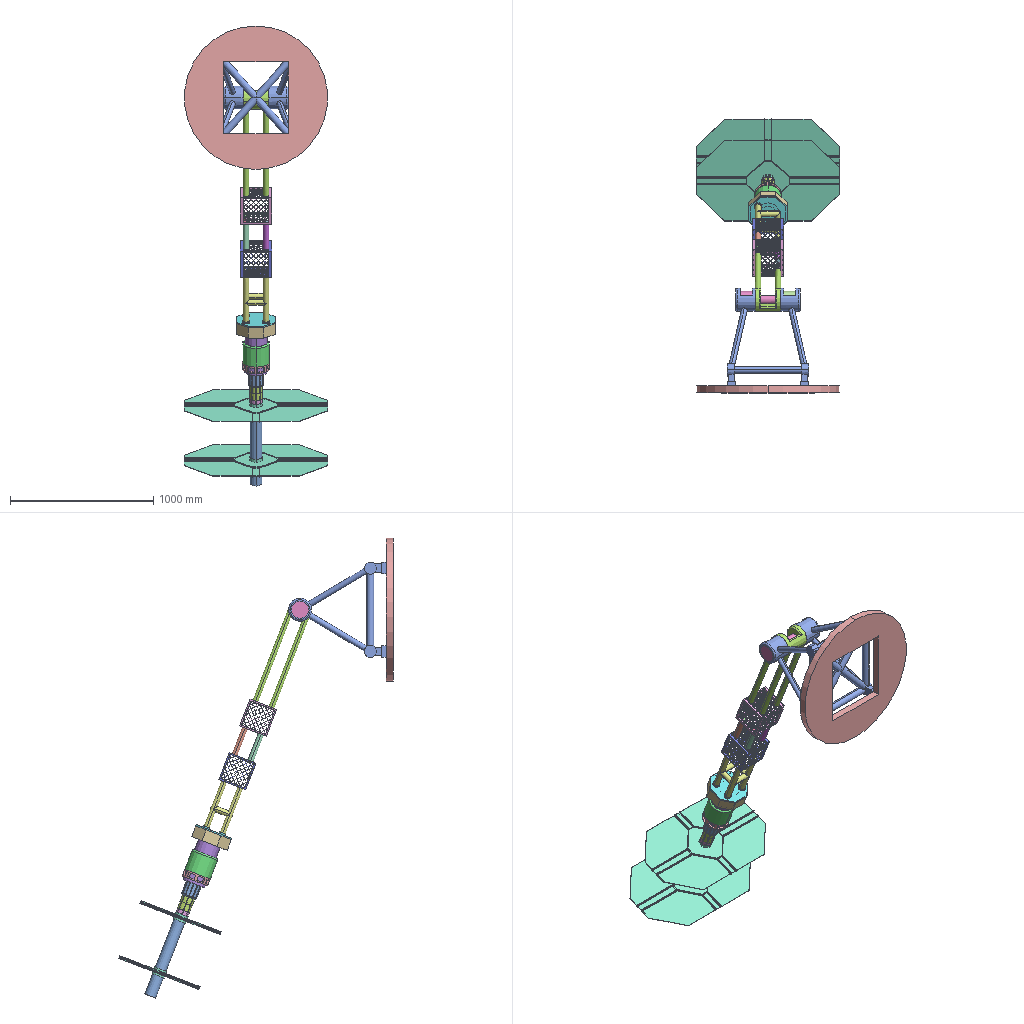Assembly | SolidWorks | 14 different items | 16 placed | box 1000 x 1914 x 3207 mm
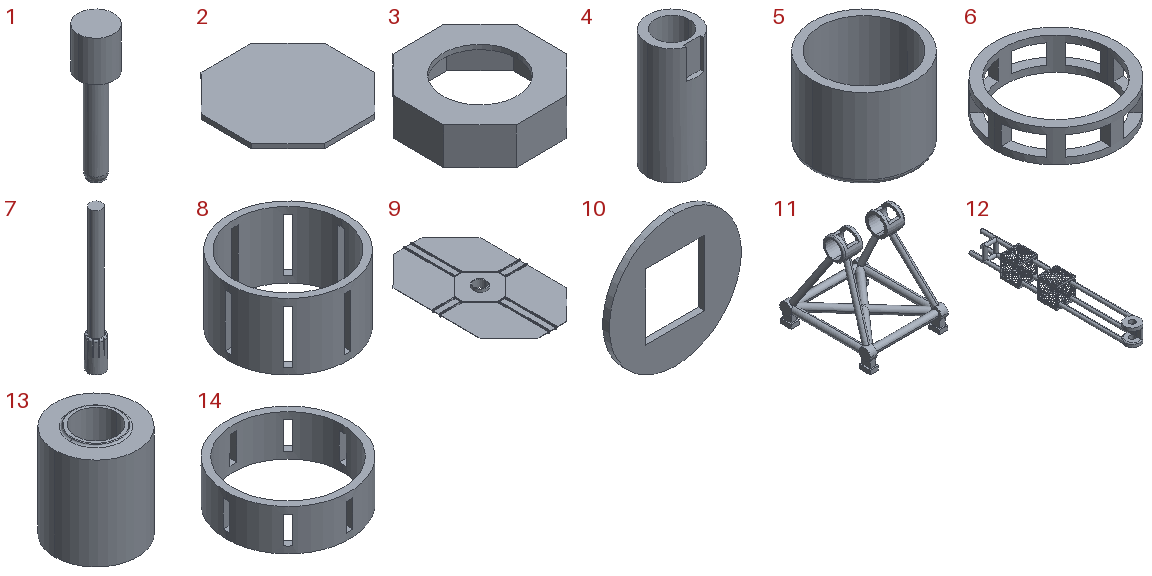Parts list (item | quantity | size | volume | features):
1 | x1 | 120 x 120 x 453 mm | 2398988 mm3 | features ICE 2, Extrusion 1, Fillet 1
2 | x1 | 265.563 x 265.563 x 20 mm | 605445 mm3 | features Extrusion 1, ICE 1
3 | x1 | 265.563 x 265.563 x 80 mm | 975982 mm3 | features Cut 1, Extrusion 1, Shell 1
4 | x1 | 160 x 160 x 380 mm | 3957629 mm3 | features Cut 2, Extrusion 1
5 | x1 | 190 x 190 x 150 mm | 1224494 mm3 | features Extrusion 1, Fillet 1
6 | x1 | 190 x 190 x 50 mm | 237092 mm3 | features Cut 1, Extrusion 1
7 | x1 | 110 x 110 x 940 mm | 5584341 mm3 | features Cut 1, Extrusion 1, Fillet 1, ICE 1
8 | x2 | 90 x 90 x 50 mm | 58754 mm3 | features CirPattern 1, Cut 1, Extrusion 1
9 | x2 | 600 x 1000 x 50 mm | 1624743 mm3 | features ICE 3, BossThin 1, Extrusion 1
10 | x1 | 1000 x 50 x 1000 mm | 28019908 mm3 | features Cut 1, Extrusion 1
11 | x1 | 570 x 664.853 x 679.884 mm | 12658453 mm3 | features ICE 6, Cut 3, Sweep 3, 3DProfileFeature 2, MirrorPattern 2, Extrusion 1, Fillet 1
12 | x1 | - | 7988146 mm3 | features ICE 8, Cut 6, BossThin 3, MirrorPattern 3, Extrusion 1, Fillet 1, LPattern 1, Sweep 1
13 | x1 | 120 x 120 x 138 mm | 1148576 mm3 | features Fillet 2, Extrusion 1, ICE 1
14 | x1 | 90 x 90 x 30 mm | 36053 mm3 | features CirPattern 1, Cut 1, Extrusion 1
Mates (type | each side: item.copy, entity, surface, feature):
InPlace | 10.1 face plane Boss-Extrude1 | 11.1 plane
Concentric | 11.1 face cylinder Cut-Extrude1 | 12.1 face cylinder Boss-Extrude1
Coincident | 11.1 face plane Cut-Extrude2 | 12.1 face plane Boss-Extrude1
Concentric | 11.1 face cylinder Cut-Extrude1 | 13.1 face cylinder Boss-Extrude1
Coincident | 11.1 face plane Boss-Extrude9 | 13.1 face plane Boss-Extrude1
Concentric | 13.1 face cylinder Boss-Extrude1 | 1.1 face cylinder Boss-Extrude2
Coincident | 11.1 face plane Boss-Extrude9 | 1.1 face plane Boss-Extrude1
InPlace | 12.1 face plane Boss-Extrude7 | 2.1 plane
InPlace | 2.1 face plane Boss-Extrude2 | 3.1 plane
InPlace | 2.1 face plane Boss-Extrude2 | 4.1 plane
Concentric | 4.1 face cylinder Boss-Extrude1 | 5.1 face cylinder Boss-Extrude1
DistanceDim | 3.1 face plane Boss-Extrude1 | 5.1 face plane Boss-Extrude1
InPlace | 5.1 face plane Boss-Extrude1 | 6.1 plane
InPlace | 4.1 face plane Boss-Extrude1 | 7.1 plane
InPlace | 7.1 face plane Boss-Extrude1 | 8.1 plane
Concentric | 8.1 face cylinder Boss-Extrude1 | 8.2 face cylinder Boss-Extrude1
Coincident | 8.1 face plane Boss-Extrude1 | 8.2 face plane Boss-Extrude1
Concentric | 8.2 face cylinder Boss-Extrude1 | 14.1 face cylinder Boss-Extrude1
Coincident | 8.2 face plane Boss-Extrude1 | 14.1 face plane Boss-Extrude1
Coincident | 8.2 face plane CirPattern1 | 14.1 face plane CirPattern1
Coincident | 8.1 face plane CirPattern1 | 8.2 face plane CirPattern1
InPlace | 14.1 face plane Boss-Extrude1 | 9.1 plane
Concentric | 7.1 face cylinder Boss-Extrude2 | 9.2 face cylinder Boss-Extrude1
DistanceDim | 9.2 face plane Boss-Extrude2 | 9.1 face plane Boss-Extrude2